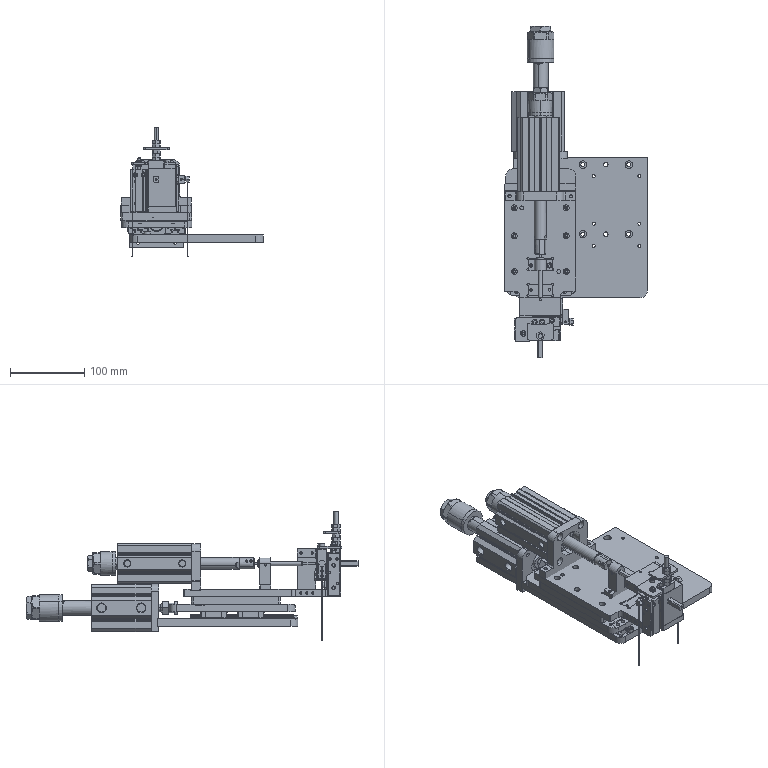Part | SolidWorks | features InContextFeatHolder 2, LocalLPattern 1, ReferencePattern 1 | 74 solids | 3271 faces | volume 1493207 mm3 | plane 1620 | cylinder 1203 | cone 368 | torus 34 | sphere 32 | spline 14 | commonest cylinder face diameters 6 x116 3.3 x102 0.4 x88 4 x83 0.8 x65 3 x58